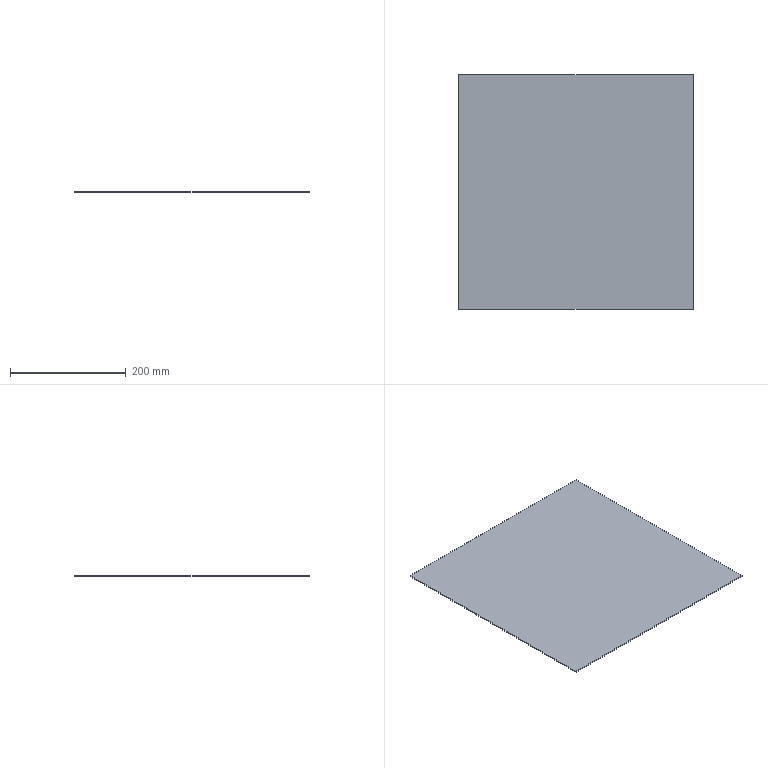Part | STEP file | 750038524 | 1 solid | 6 faces | box 405 x 405 x 1.5 mm | volume 246038 mm3 | plane 6
STEP:
#1=CARTESIAN_POINT('',(-202.5,-202.5,1.5));
#2=VERTEX_POINT('',#1);
#3=CARTESIAN_POINT('',(202.5,-202.5,1.5));
#4=VERTEX_POINT('',#3);
#5=CARTESIAN_POINT('',(0.,-202.5,1.5));
#6=DIRECTION('',(1.,0.,0.));
#7=VECTOR('',#6,1000.);
#8=LINE('',#5,#7);
#9=EDGE_CURVE('',#2,#4,#8,.T.);
#10=ORIENTED_EDGE('',*,*,#9,.T.);
#11=CARTESIAN_POINT('',(202.5,202.5,1.5));
#12=VERTEX_POINT('',#11);
#13=CARTESIAN_POINT('',(202.5,0.,1.5));
#14=DIRECTION('',(0.,1.,0.));
#15=VECTOR('',#14,1000.);
#16=LINE('',#13,#15);
#17=EDGE_CURVE('',#4,#12,#16,.T.);
#18=ORIENTED_EDGE('',*,*,#17,.T.);
#19=CARTESIAN_POINT('',(-202.5,202.5,1.5));
#20=VERTEX_POINT('',#19);
#21=CARTESIAN_POINT('',(0.,202.5,1.5));
#22=DIRECTION('',(-1.,0.,0.));
#23=VECTOR('',#22,1000.);
#24=LINE('',#21,#23);
#25=EDGE_CURVE('',#12,#20,#24,.T.);
#26=ORIENTED_EDGE('',*,*,#25,.T.);
#27=CARTESIAN_POINT('',(-202.5,0.,1.5));
#28=DIRECTION('',(0.,-1.,0.));
#29=VECTOR('',#28,1000.);
#30=LINE('',#27,#29);
#31=EDGE_CURVE('',#20,#2,#30,.T.);
#32=ORIENTED_EDGE('',*,*,#31,.T.);
#33=EDGE_LOOP('',(#10,#18,#26,#32));
#34=FACE_OUTER_BOUND('',#33,.T.);
#35=CARTESIAN_POINT('',(0.,0.,1.5));
#36=DIRECTION('',(0.,0.,1.));
#37=DIRECTION('',(1.,0.,0.));
#38=AXIS2_PLACEMENT_3D('',#35,#36,#37);
#39=PLANE('',#38);
#40=ADVANCED_FACE('',(#34),#39,.T.);
#41=CARTESIAN_POINT('',(202.5,202.5,0.));
#42=VERTEX_POINT('',#41);
#43=CARTESIAN_POINT('',(202.5,202.5,1.5));
#44=DIRECTION('',(0.,0.,-1.));
#45=VECTOR('',#44,1000.);
#46=LINE('',#43,#45);
#47=EDGE_CURVE('',#12,#42,#46,.T.);
#48=ORIENTED_EDGE('',*,*,#47,.F.);
#49=ORIENTED_EDGE('',*,*,#17,.F.);
#50=CARTESIAN_POINT('',(202.5,-202.5,0.));
#51=VERTEX_POINT('',#50);
#52=CARTESIAN_POINT('',(202.5,-202.5,1.5));
#53=DIRECTION('',(0.,0.,1.));
#54=VECTOR('',#53,1000.);
#55=LINE('',#52,#54);
#56=EDGE_CURVE('',#51,#4,#55,.T.);
#57=ORIENTED_EDGE('',*,*,#56,.F.);
#58=CARTESIAN_POINT('',(202.5,-202.5,0.));
#59=DIRECTION('',(0.,-1.,0.));
#60=VECTOR('',#59,1000.);
#61=LINE('',#58,#60);
#62=EDGE_CURVE('',#42,#51,#61,.T.);
#63=ORIENTED_EDGE('',*,*,#62,.F.);
#64=EDGE_LOOP('',(#48,#49,#57,#63));
#65=FACE_OUTER_BOUND('',#64,.T.);
#66=CARTESIAN_POINT('',(202.5,-202.5,1.5));
#67=DIRECTION('',(-1.,0.,0.));
#68=DIRECTION('',(0.,0.,1.));
#69=AXIS2_PLACEMENT_3D('',#66,#67,#68);
#70=PLANE('',#69);
#71=ADVANCED_FACE('',(#65),#70,.F.);
#72=ORIENTED_EDGE('',*,*,#56,.T.);
#73=ORIENTED_EDGE('',*,*,#9,.F.);
#74=CARTESIAN_POINT('',(-202.5,-202.5,0.));
#75=VERTEX_POINT('',#74);
#76=CARTESIAN_POINT('',(-202.5,-202.5,1.5));
#77=DIRECTION('',(0.,0.,1.));
#78=VECTOR('',#77,1000.);
#79=LINE('',#76,#78);
#80=EDGE_CURVE('',#75,#2,#79,.T.);
#81=ORIENTED_EDGE('',*,*,#80,.F.);
#82=CARTESIAN_POINT('',(-202.5,-202.5,0.));
#83=DIRECTION('',(-1.,0.,0.));
#84=VECTOR('',#83,1000.);
#85=LINE('',#82,#84);
#86=EDGE_CURVE('',#51,#75,#85,.T.);
#87=ORIENTED_EDGE('',*,*,#86,.F.);
#88=EDGE_LOOP('',(#72,#73,#81,#87));
#89=FACE_OUTER_BOUND('',#88,.T.);
#90=CARTESIAN_POINT('',(-202.5,-202.5,1.5));
#91=DIRECTION('',(0.,1.,0.));
#92=DIRECTION('',(0.,0.,1.));
#93=AXIS2_PLACEMENT_3D('',#90,#91,#92);
#94=PLANE('',#93);
#95=ADVANCED_FACE('',(#89),#94,.F.);
#96=ORIENTED_EDGE('',*,*,#80,.T.);
#97=ORIENTED_EDGE('',*,*,#31,.F.);
#98=CARTESIAN_POINT('',(-202.5,202.5,0.));
#99=VERTEX_POINT('',#98);
#100=CARTESIAN_POINT('',(-202.5,202.5,1.5));
#101=DIRECTION('',(0.,0.,1.));
#102=VECTOR('',#101,1000.);
#103=LINE('',#100,#102);
#104=EDGE_CURVE('',#99,#20,#103,.T.);
#105=ORIENTED_EDGE('',*,*,#104,.F.);
#106=CARTESIAN_POINT('',(-202.5,202.5,0.));
#107=DIRECTION('',(0.,1.,0.));
#108=VECTOR('',#107,1000.);
#109=LINE('',#106,#108);
#110=EDGE_CURVE('',#75,#99,#109,.T.);
#111=ORIENTED_EDGE('',*,*,#110,.F.);
#112=EDGE_LOOP('',(#96,#97,#105,#111));
#113=FACE_OUTER_BOUND('',#112,.T.);
#114=CARTESIAN_POINT('',(-202.5,202.5,1.5));
#115=DIRECTION('',(1.,0.,0.));
#116=DIRECTION('',(0.,0.,-1.));
#117=AXIS2_PLACEMENT_3D('',#114,#115,#116);
#118=PLANE('',#117);
#119=ADVANCED_FACE('',(#113),#118,.F.);
#120=ORIENTED_EDGE('',*,*,#104,.T.);
#121=ORIENTED_EDGE('',*,*,#25,.F.);
#122=ORIENTED_EDGE('',*,*,#47,.T.);
#123=CARTESIAN_POINT('',(202.5,202.5,0.));
#124=DIRECTION('',(1.,0.,0.));
#125=VECTOR('',#124,1000.);
#126=LINE('',#123,#125);
#127=EDGE_CURVE('',#99,#42,#126,.T.);
#128=ORIENTED_EDGE('',*,*,#127,.F.);
#129=EDGE_LOOP('',(#120,#121,#122,#128));
#130=FACE_OUTER_BOUND('',#129,.T.);
#131=CARTESIAN_POINT('',(202.5,202.5,1.5));
#132=DIRECTION('',(0.,-1.,0.));
#133=DIRECTION('',(0.,0.,-1.));
#134=AXIS2_PLACEMENT_3D('',#131,#132,#133);
#135=PLANE('',#134);
#136=ADVANCED_FACE('',(#130),#135,.F.);
#137=ORIENTED_EDGE('',*,*,#62,.T.);
#138=ORIENTED_EDGE('',*,*,#86,.T.);
#139=ORIENTED_EDGE('',*,*,#110,.T.);
#140=ORIENTED_EDGE('',*,*,#127,.T.);
#141=EDGE_LOOP('',(#137,#138,#139,#140));
#142=FACE_OUTER_BOUND('',#141,.T.);
#143=CARTESIAN_POINT('',(0.,0.,0.));
#144=DIRECTION('',(0.,0.,1.));
#145=DIRECTION('',(1.,0.,0.));
#146=AXIS2_PLACEMENT_3D('',#143,#144,#145);
#147=PLANE('',#146);
#148=ADVANCED_FACE('',(#142),#147,.F.);
#149=CLOSED_SHELL('',(#40,#71,#95,#119,#136,#148));
#150=MANIFOLD_SOLID_BREP('',#149);
#151=CARTESIAN_POINT('',(0.,0.,0.));
#152=DIRECTION('',(0.,0.,1.));
#153=DIRECTION('',(1.,0.,0.));
#154=AXIS2_PLACEMENT_3D('',#151,#152,#153);
#155=(LENGTH_UNIT()NAMED_UNIT(*)SI_UNIT(.MILLI.,.METRE.));
#156=UNCERTAINTY_MEASURE_WITH_UNIT(LENGTH_MEASURE(0.00001),#155,'','');
#157=(NAMED_UNIT(*)PLANE_ANGLE_UNIT()SI_UNIT($,.RADIAN.));
#158=(NAMED_UNIT(*)SI_UNIT($,.STERADIAN.)SOLID_ANGLE_UNIT());
#159=(GEOMETRIC_REPRESENTATION_CONTEXT(3)GLOBAL_UNCERTAINTY_ASSIGNED_CONTEXT((#156))GLOBAL_UNIT_ASSIGNED_CONTEXT((#155,#157,#158))REPRESENTATION_CONTEXT('',''));
#160=ADVANCED_BREP_SHAPE_REPRESENTATION('',(#150,#154),#159);